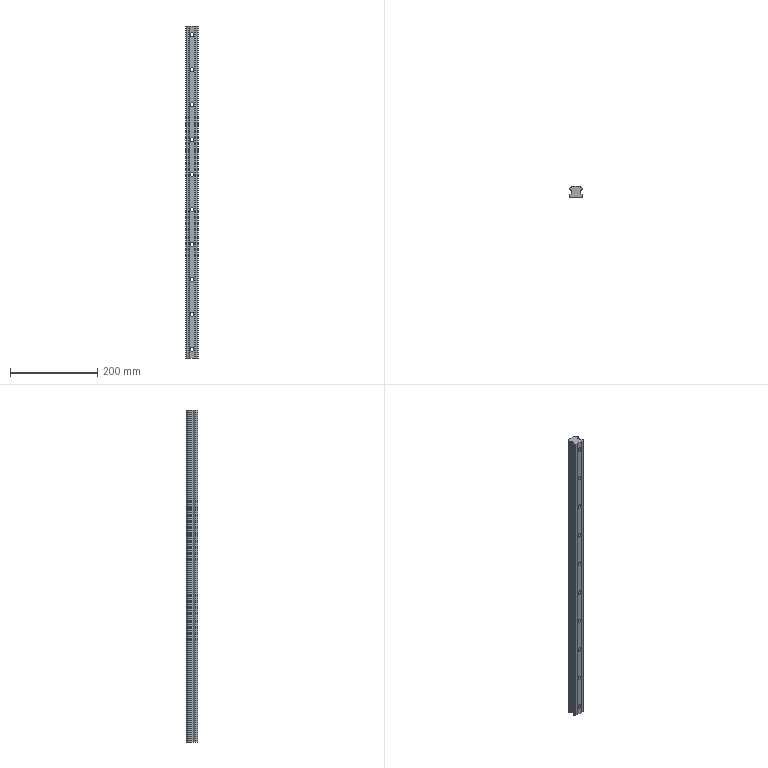Part | STEP file | HGR30R-760 Slide Rail | 1 solid | 102 faces | box 28 x 26 x 760 mm | volume 438693 mm3 | cylinder 62 | plane 40 | commonest cylinder face diameters 9 x20 14 x20 1.2 x12 1.6 x6 5.66 x4